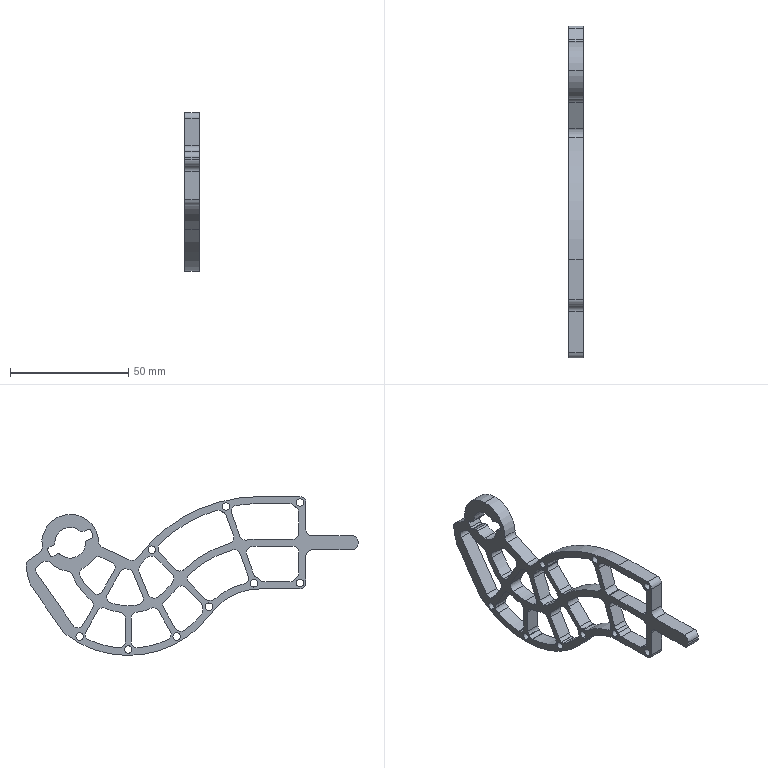Part | SolidWorks | features Fillet 2, Extrusion 1, ICE 1 | 1 solid | 199 faces | box 6 x 140.191 x 67.073 mm | volume 12197 mm3 | cylinder 154 | plane 45 | commonest cylinder face diameters 5 x84 3.2 x18 2 x10 5.5 x9 51 x5 24 x4